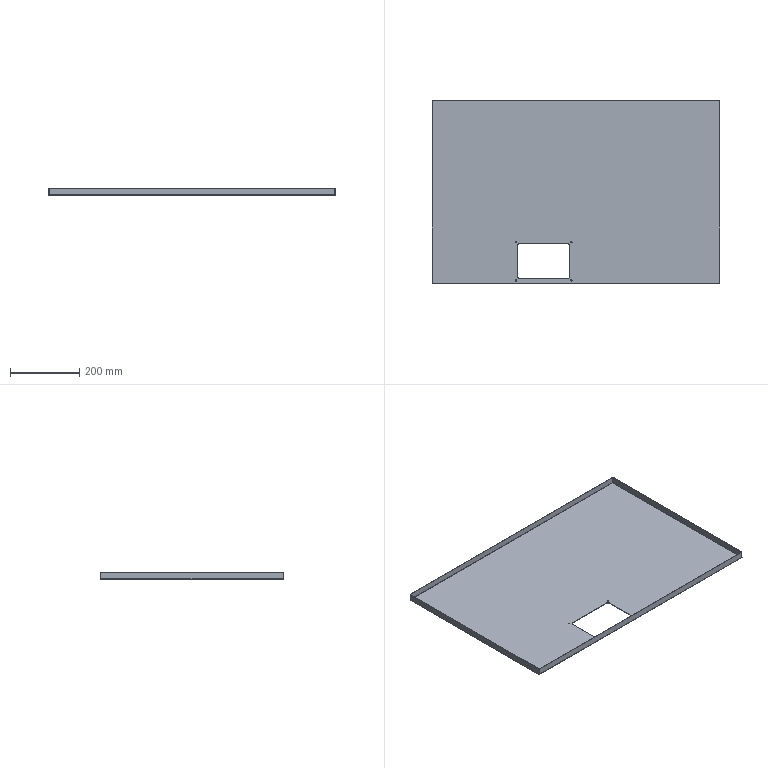Part | SolidWorks | 1 solid | 54 faces | box 830.001 x 530.001 x 20 mm | volume 710788 mm3 | plane 26 | cylinder 20 | spline 8 | commonest cylinder face diameters 4.2 x8 0.2 x4 3.2 x4 10 x4